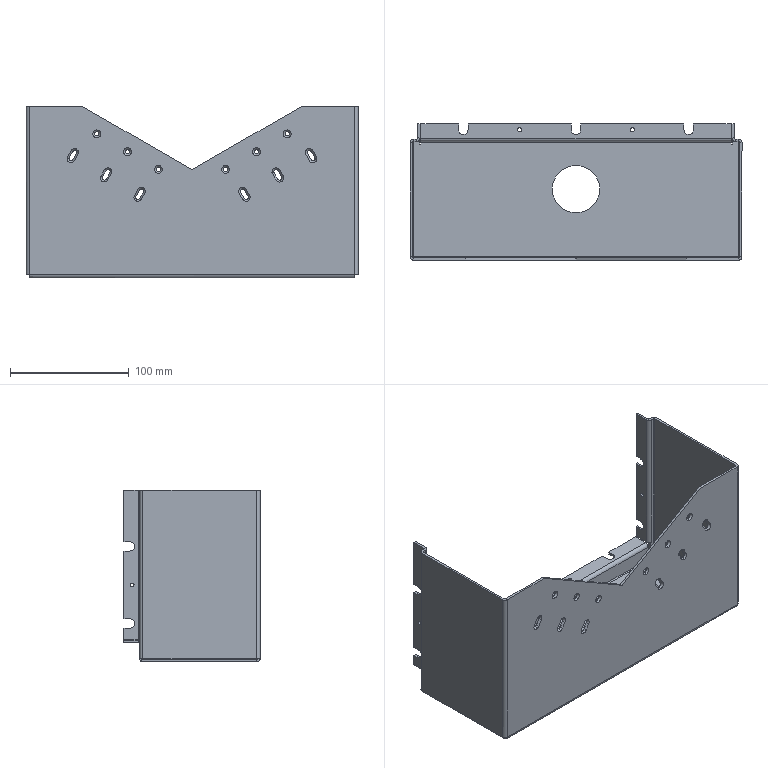Part | SolidWorks | features Cut 7, EdgeFlange 7, Fillet 2, MirrorPattern 2, Chamfer 1, FlatPattern 1, HoleWzd 1, ICE 1, SMBaseFlange 1, SheetMetal 1, SketchPattern 1 | 1 solid | 224 faces | box 280 x 115 x 145 mm | volume 201442 mm3 | plane 120 | cylinder 70 | cone 30 | spline 4 | commonest cylinder face diameters 3.6 x30 8 x11 2 x10 6 x9 3.2 x4 3.5 x4